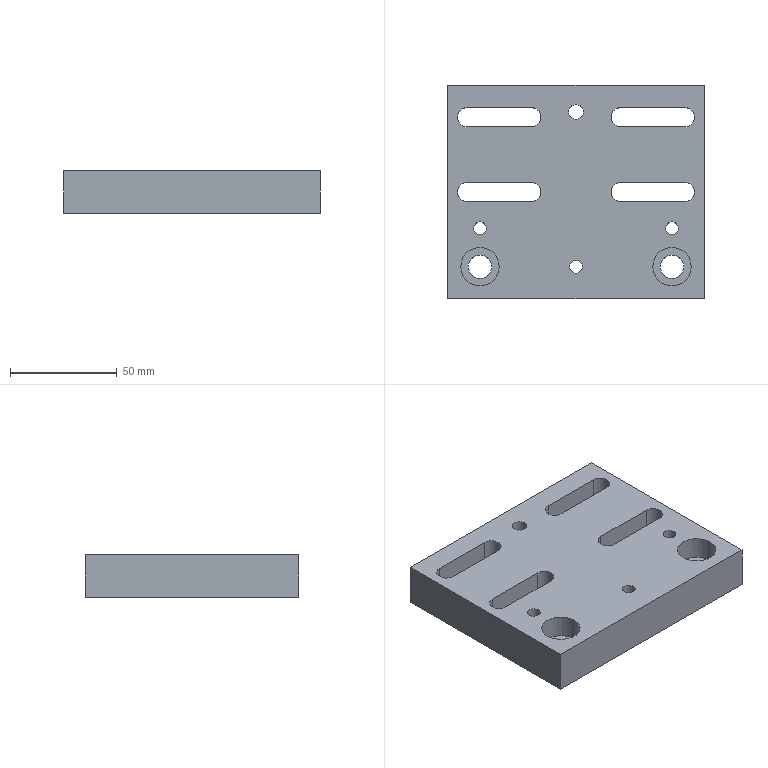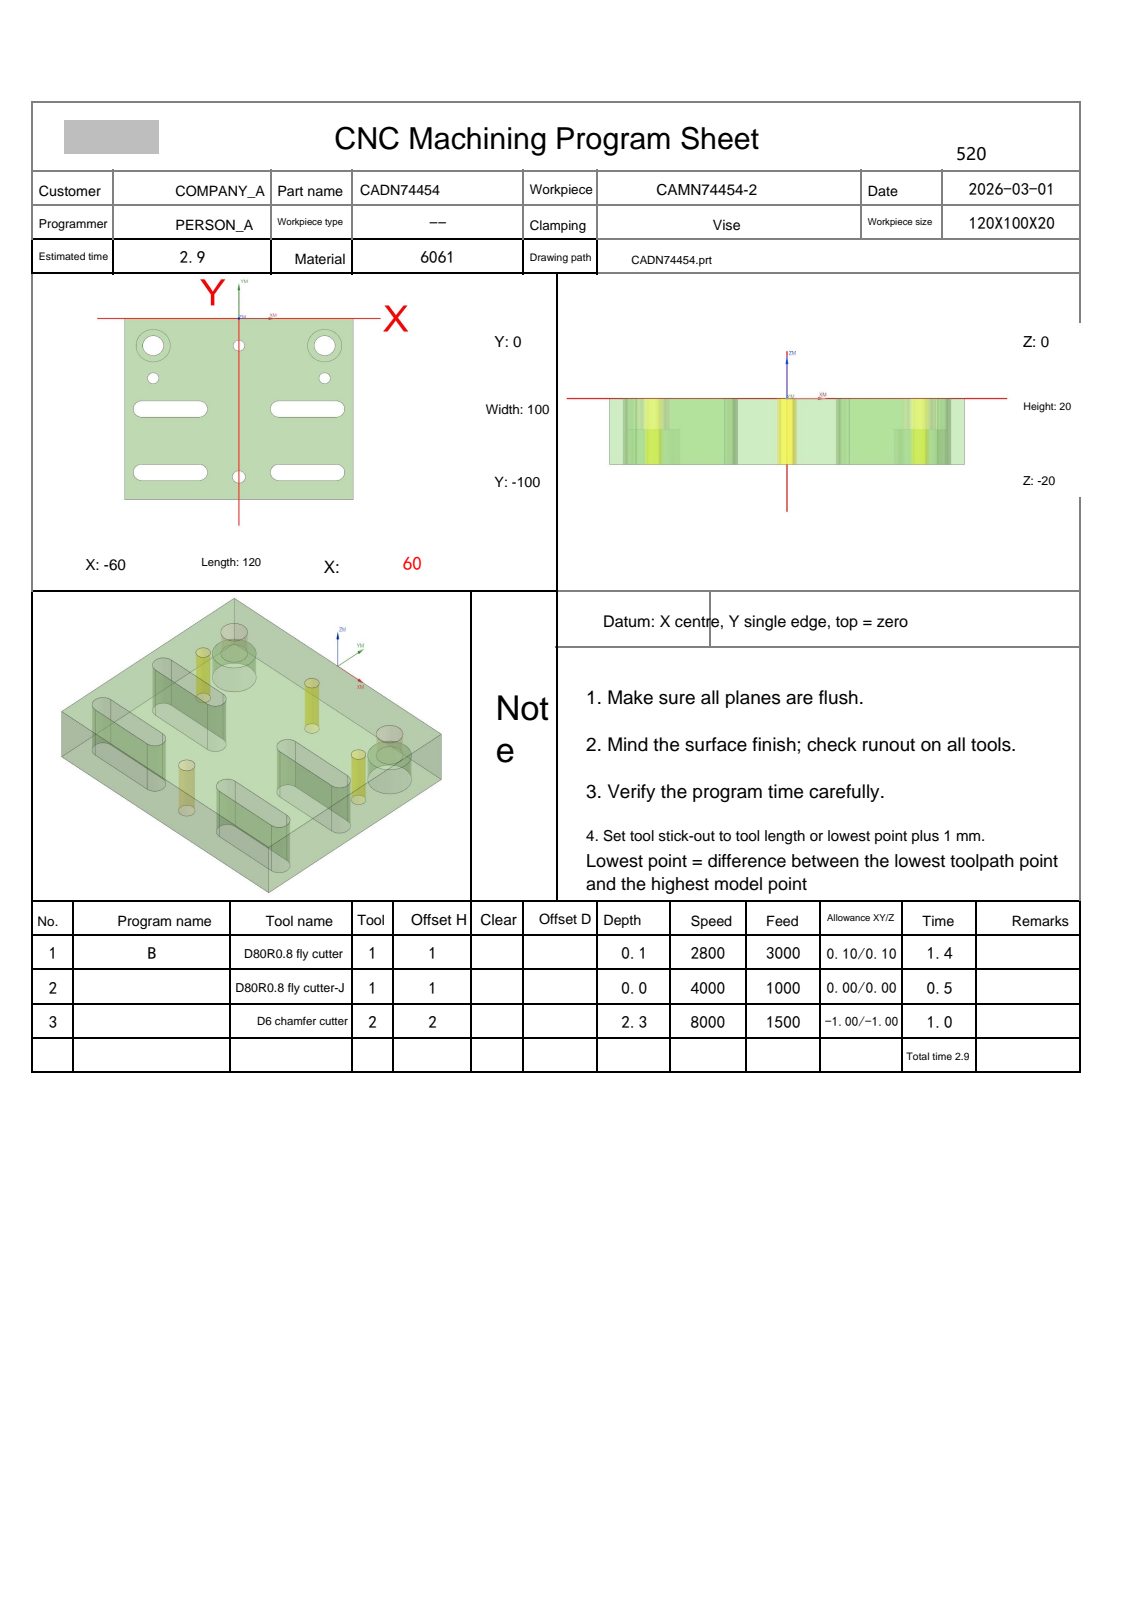NC program | NX | posted by the shop | part box 120 x 100 x 20 mm
Whole program:
%
O0001
(Machine time: 3.45 MIN)
(===Total Tool:2===)
(T1=D80R0.8 fly cutter D=80.  R=0.8  D-  H01 Z=0.    )
(T2=D6 chamfer cutter   D=6.   R=0.   D-  H02 Z=-2.3  )
G80 G90 G17 G49 G40
G91 G28 Z0
M01
N1 T01 M06
(D80R0.8 fly cutter  D=80. R=0.8 H=01 ce=0.10 di=0.10)
G00 G90 G54 X112.097 Y-76.097 M03 S2800
G43 H01 Z50.
M08
Z6.011
G01 Z4.011 F3000.
X100.097
X-92.897
G02 X-100.097 Y-68.897 I0.0 J7.2
G01 Y-39.263
G02 X-92.097 Y-31.263 I8. J0.0
G01 X100.097
X112.097
Z6.011
G00 Y-76.097
Z5.522
G01 Z3.522
X100.097
X-92.897
G02 X-100.097 Y-68.897 I0.0 J7.2
G01 Y-39.263
G02 X-92.097 Y-31.263 I8. J0.0
G01 X100.097
X112.097
Z5.522
G00 Y-76.097
Z5.033
G01 Z3.033
X100.097
X-92.897
G02 X-100.097 Y-68.897 I0.0 J7.2
G01 Y-39.263
G02 X-92.097 Y-31.263 I8. J0.0
G01 X100.097
X112.097
Z5.033
G00 Y-76.097
Z4.544
G01 Z2.544
X100.097
X-92.897
G02 X-100.097 Y-68.897 I0.0 J7.2
G01 Y-39.263
G02 X-92.097 Y-31.263 I8. J0.0
G01 X100.097
X112.097
Z4.544
G00 Y-76.097
Z4.056
G01 Z2.056
X100.097
X-92.897
G02 X-100.097 Y-68.897 I0.0 J7.2
G01 Y-39.263
G02 X-92.097 Y-31.263 I8. J0.0
G01 X100.097
X112.097
Z4.056
G00 Y-76.097
Z3.567
G01 Z1.567
X100.097
X-92.897
G02 X-100.097 Y-68.897 I0.0 J7.2
G01 Y-39.263
G02 X-92.097 Y-31.263 I8. J0.0
G01 X100.097
X112.097
Z3.567
G00 Y-76.097
Z3.078
G01 Z1.078
X100.097
X-92.897
G02 X-100.097 Y-68.897 I0.0 J7.2
G01 Y-39.263
G02 X-92.097 Y-31.263 I8. J0.0
G01 X100.097
X112.097
Z3.078
G00 Y-76.097
Z2.589
G01 Z.589
X100.097
X-92.897
G02 X-100.097 Y-68.897 I0.0 J7.2
G01 Y-39.263
G02 X-92.097 Y-31.263 I8. J0.0
G01 X100.097
X112.097
Z2.589
G00 Y-76.097
Z2.1
G01 Z.1
X100.097
X-92.897
G02 X-100.097 Y-68.897 I0.0 J7.2
G01 Y-39.263
G02 X-92.097 Y-31.263 I8. J0.0
G01 X100.097
X112.097
Z2.1
G00 Z50.
G91 G28 Z0.0
M05
M09
G91 G28 Z0.0
M01
N2 T01 M06
(D80R0.8 fly cutter-J  D=80. R=0.8 H=01 ce=0.00 di=0.00)
G00 G90 G54 X111.999 Y-75.999 M03 S4000
G43 H01 Z50.
M08
Z2.
G01 Z0.0 F1000.
X99.999
X-92.799
G02 X-99.999 Y-68.799 I0.0 J7.2
G01 Y-39.361
G02 X-91.999 Y-31.361 I8. J0.0
G01 X99.999
X111.999
Z2.
G00 Z50.
G91 G28 Z0.0
M05
M09
G91 G28 Z0.0
M01
N3 T02 M06
(D6 chamfer cutter  D=6. R=0. H=02 ce=-0.30 di=-0.80)
G00 G90 G54 X45.232 Y-33.87 M03 S8000
G43 H02 Z50.
M08
Z-.9
G01 Z-1.4 F600.
X45.4 Y-34.5
G03 X46.9 Y-33. I0.0 J1.5
X45. Y-31.1 I-1.9 J0.0
X43.1 Y-33. I0.0 J-1.9
X45. Y-34.9 I1.9 J0.0
X46.9 Y-33. I0.0 J1.9
X45.4 Y-31.5 I-1.5 J0.0
G01 X45.232 Y-32.13
Z-.9
G00 Z50.
X.232 Y-15.87
Z-.9
G01 Z-1.4
X.4 Y-16.5
G03 X1.9 Y-15. I0.0 J1.5
X0.0 Y-13.1 I-1.9 J0.0
X-1.9 Y-15. I0.0 J-1.9
X0.0 Y-16.9 I1.9 J0.0
X1.9 Y-15. I0.0 J1.9
X.4 Y-13.5 I-1.5 J0.0
G01 X.232 Y-14.13
Z-.9
G00 Z50.
X-44.768 Y-33.87
Z-.9
G01 Z-1.4
X-44.6 Y-34.5
G03 X-43.1 Y-33. I0.0 J1.5
X-45. Y-31.1 I-1.9 J0.0
X-46.9 Y-33. I0.0 J-1.9
X-45. Y-34.9 I1.9 J0.0
X-43.1 Y-33. I0.0 J1.9
X-44.6 Y-31.5 I-1.5 J0.0
G01 X-44.768 Y-32.13
Z-.9
G00 Z50.
G00 G90 X0.0 Y-89.5 M03 S8000
Z50.
Z-.9
G01 Z-1.4 F600.
Y-90.5
G03 X3. Y-87.5 I0.0 J3.
X0.0 Y-84.5 I-3. J0.0
X-3. Y-87.5 I0.0 J-3.
X0.0 Y-90.5 I3. J0.0
X3. Y-87.5 I0.0 J3.
X0.0 Y-84.5 I-3. J0.0
G01 Y-85.5
Z-.9
G00 Z50.
G00 G90 X44.589 Y-12.534 M03 S8000
Z50.
Z-1.8
G01 Z-2.3 F1200.
X44.5 Y-12.
G03 X41.5 Y-15. I0.0 J-3.
X45. Y-18.5 I3.5 J0.0
X48.5 Y-15. I0.0 J3.5
X45. Y-11.5 I-3.5 J0.0
X41.5 Y-15. I0.0 J-3.5
X44.5 Y-18. I3. J0.0
G01 X44.589 Y-17.466
Z-1.8
G00 Z50.
X-45.411 Y-12.534
Z-1.8
G01 Z-2.3
X-45.5 Y-12.
G03 X-48.5 Y-15. I0.0 J-3.
X-45. Y-18.5 I3.5 J0.0
X-41.5 Y-15. I0.0 J3.5
X-45. Y-11.5 I-3.5 J0.0
X-48.5 Y-15. I0.0 J-3.5
X-45.5 Y-18. I3. J0.0
G01 X-45.411 Y-17.466
Z-1.8
G00 Z50.
G00 G90 X.386 Y-101.227 M03 S6500
Z50.
Z.172
G01 Z-1.2 F1500.
G03 X.1 Y-101.027 I-1.286 J-1.532
G01 X.054 Y-100.997
X0.0 Y-101.
X-60.
G02 X-61. Y-100. I0.0 J1.
G01 Y0.0
G02 X-60. Y1. I1. J0.0
G01 X60.
G02 X61. Y0.0 I0.0 J-1.
G01 Y-100.
G02 X60. Y-101. I-1. J0.0
G01 X0.0
X-.054 Y-100.997
X-.1 Y-101.027
G03 X-.386 Y-101.227 I1. J-1.732
G01 Z.172
G00 Z10.
X-49.299 Y-14.6
Z.224
G01 Z-1.2
G03 X-49.48 Y-14.898 I1.613 J-1.183
G01 X-49.506 Y-14.946
X-49.5 Y-15.
G03 X-45. Y-19.5 I4.5 J0.0
X-40.5 Y-15. I0.0 J4.5
X-45. Y-10.5 I-4.5 J0.0
X-49.5 Y-15. I0.0 J-4.5
G01 X-49.506 Y-15.054
X-49.48 Y-15.102
G03 X-49.299 Y-15.4 I1.794 J.885
G01 Z.224
G00 Z10.
X-43.192 Y-33.404
Z.257
G01 Z-1.2
G03 X-43.018 Y-33.102 I-1.638 J1.147
G01 X-42.992 Y-33.054
X-43. Y-33.
G03 X-45. Y-31. I-2. J0.0
X-47. Y-33. I0.0 J-2.
X-45. Y-35. I2. J0.0
X-43.03 Y-33.347 I0.0 J2.
G01 X-43. Y-33.
X-42.992 Y-32.946
X-43.018 Y-32.898
G03 X-43.192 Y-32.596 I-1.813 J-.845
G01 Z.257
G00 Z10.
X-35.614 Y-46.727
Z.172
G01 Z-1.2
G03 X-35.9 Y-46.527 I-1.286 J-1.532
G01 X-35.946 Y-46.497
X-36. Y-46.5
X-51.
G03 X-54.5 Y-50. I0.0 J-3.5
X-51. Y-53.5 I3.5 J0.0
G01 X-21.
G03 X-17.5 Y-50. I0.0 J3.5
X-21. Y-46.5 I-3.5 J0.0
G01 X-36.
X-36.054 Y-46.497
X-36.1 Y-46.527
G03 X-36.386 Y-46.727 I1. J-1.732
G01 Z.172
G00 Z10.
X-35.614 Y-81.727
Z.172
G01 Z-1.2
G03 X-35.9 Y-81.527 I-1.286 J-1.532
G01 X-35.946 Y-81.497
X-36. Y-81.5
X-51.
G03 X-54.5 Y-85. I0.0 J-3.5
X-51. Y-88.5 I3.5 J0.0
G01 X-21.
G03 X-17.5 Y-85. I0.0 J3.5
X-21. Y-81.5 I-3.5 J0.0
G01 X-36.
X-36.054 Y-81.497
X-36.1 Y-81.527
G03 X-36.386 Y-81.727 I1. J-1.732
G01 Z.172
G00 Z10.
X2.208 Y-87.904
Z.252
G01 Z-1.2
G03 X2.382 Y-87.602 I-1.638 J1.147
G01 X2.408 Y-87.554
X2.4 Y-87.5
G03 X0.0 Y-85.1 I-2.4 J0.0
X-2.4 Y-87.5 I0.0 J-2.4
X0.0 Y-89.9 I2.4 J0.0
X2.4 Y-87.5 I0.0 J2.4
G01 X2.408 Y-87.446
X2.382 Y-87.398
G03 X2.208 Y-87.096 I-1.813 J-.845
G01 Z.252
G00 Z10.
X35.614 Y-88.273
Z.172
G01 Z-1.2
G03 X35.9 Y-88.473 I1.286 J1.532
G01 X35.946 Y-88.503
X36. Y-88.5
X51.
G03 X54.5 Y-85. I0.0 J3.5
X51. Y-81.5 I-3.5 J0.0
G01 X21.
G03 X17.5 Y-85. I0.0 J-3.5
X21. Y-88.5 I3.5 J0.0
G01 X36.
X36.054 Y-88.503
X36.1 Y-88.473
G03 X36.386 Y-88.273 I-1. J1.732
G01 Z.172
G00 Z10.
X35.614 Y-53.273
Z.172
G01 Z-1.2
G03 X35.9 Y-53.473 I1.286 J1.532
G01 X35.946 Y-53.503
X36. Y-53.5
X51.
G03 X54.5 Y-50. I0.0 J3.5
X51. Y-46.5 I-3.5 J0.0
G01 X21.
G03 X17.5 Y-50. I0.0 J-3.5
X21. Y-53.5 I3.5 J0.0
G01 X36.
X36.054 Y-53.503
X36.1 Y-53.473
G03 X36.386 Y-53.273 I-1. J1.732
G01 Z.172
G00 Z10.
X46.808 Y-33.404
Z.257
G01 Z-1.2
G03 X46.982 Y-33.102 I-1.638 J1.147
G01 X47.008 Y-33.054
X47. Y-33.
G03 X45. Y-31. I-2. J0.0
X43. Y-33. I0.0 J-2.
X45. Y-35. I2. J0.0
X46.97 Y-33.347 I0.0 J2.
G01 X47. Y-33.
X47.008 Y-32.946
X46.982 Y-32.898
G03 X46.808 Y-32.596 I-1.813 J-.845
G01 Z.257
G00 Z10.
X40.701 Y-14.6
Z.224
G01 Z-1.2
G03 X40.52 Y-14.898 I1.613 J-1.183
G01 X40.494 Y-14.946
X40.5 Y-15.
G03 X45. Y-19.5 I4.5 J0.0
X49.5 Y-15. I0.0 J4.5
X45. Y-10.5 I-4.5 J0.0
X40.5 Y-15. I0.0 J-4.5
G01 X40.494 Y-15.054
X40.52 Y-15.102
G03 X40.701 Y-15.4 I1.794 J.885
G01 Z.224
G00 Z10.
X1.808 Y-15.404
Z.257
G01 Z-1.2
G03 X1.982 Y-15.102 I-1.638 J1.147
G01 X2.008 Y-15.054
X2. Y-15.
G03 X0.0 Y-13. I-2. J0.0
X-2. Y-15. I0.0 J-2.
X0.0 Y-17. I2. J0.0
X1.97 Y-15.347 I0.0 J2.
G01 X2. Y-15.
X2.008 Y-14.946
X1.982 Y-14.898
G03 X1.808 Y-14.596 I-1.813 J-.845
G01 Z.257
G00 Z50.
M05
M09
G91 G28 Z0.0
G91 G28 Y0.0
M30
%